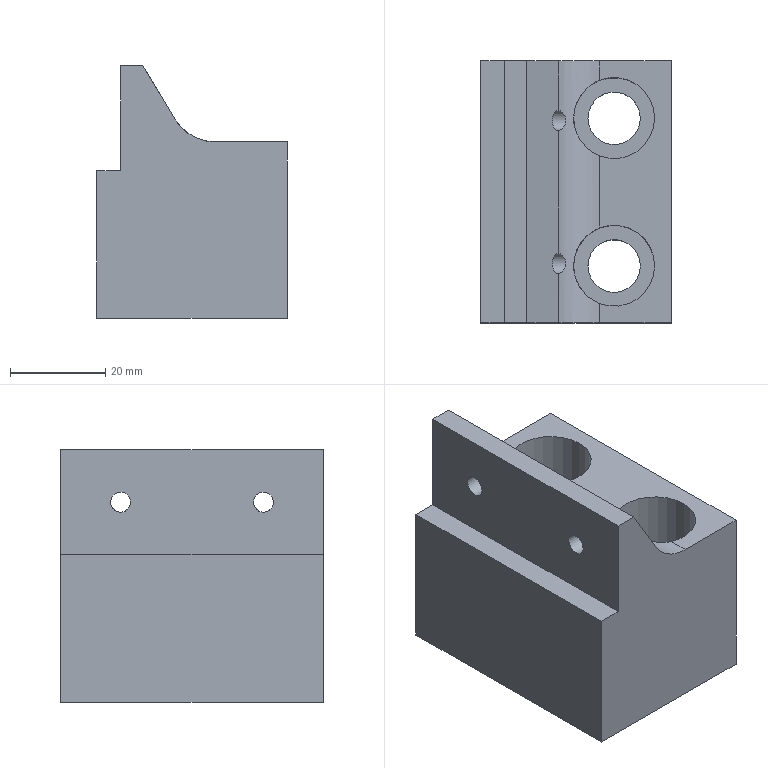Part | STEP file | 1 solid | 19 faces | box 40 x 55 x 53 mm | volume 73845 mm3 | plane 12 | cylinder 7 | commonest cylinder face diameters 4.2 x2 11 x2 17 x2 20 x1
STEP:
#1=CARTESIAN_POINT('',(132.93,-48.426,-20.));
#2=VERTEX_POINT('',#1);
#3=CARTESIAN_POINT('',(132.93,-32.574,-20.));
#4=VERTEX_POINT('',#3);
#5=CARTESIAN_POINT('',(136.,-40.5,-20.));
#6=DIRECTION('',(0.,0.,1.));
#7=DIRECTION('',(-1.,0.,0.));
#8=AXIS2_PLACEMENT_3D('',#5,#6,#7);
#9=CIRCLE('',#8,8.5);
#10=EDGE_CURVE('',#2,#4,#9,.T.);
#11=ORIENTED_EDGE('',*,*,#10,.F.);
#12=CARTESIAN_POINT('',(132.93,-63.574,-20.));
#13=VERTEX_POINT('',#12);
#14=CARTESIAN_POINT('',(132.93,-56.,-20.));
#15=DIRECTION('',(0.,-1.,0.));
#16=VECTOR('',#15,1.);
#17=LINE('',#14,#16);
#18=EDGE_CURVE('',#2,#13,#17,.T.);
#19=ORIENTED_EDGE('',*,*,#18,.T.);
#20=CARTESIAN_POINT('',(132.93,-79.426,-20.));
#21=VERTEX_POINT('',#20);
#22=CARTESIAN_POINT('',(136.,-71.5,-20.));
#23=DIRECTION('',(0.,0.,-1.));
#24=DIRECTION('',(-1.,0.,0.));
#25=AXIS2_PLACEMENT_3D('',#22,#23,#24);
#26=CIRCLE('',#25,8.5);
#27=EDGE_CURVE('',#13,#21,#26,.T.);
#28=ORIENTED_EDGE('',*,*,#27,.T.);
#29=CARTESIAN_POINT('',(132.93,-83.5,-20.));
#30=VERTEX_POINT('',#29);
#31=CARTESIAN_POINT('',(132.93,-56.,-20.));
#32=DIRECTION('',(0.,-1.,0.));
#33=VECTOR('',#32,1.);
#34=LINE('',#31,#33);
#35=EDGE_CURVE('',#21,#30,#34,.T.);
#36=ORIENTED_EDGE('',*,*,#35,.T.);
#37=CARTESIAN_POINT('',(148.,-83.5,-20.));
#38=VERTEX_POINT('',#37);
#39=CARTESIAN_POINT('',(106.5,-83.5,-20.));
#40=DIRECTION('',(-1.,0.,0.));
#41=VECTOR('',#40,1.);
#42=LINE('',#39,#41);
#43=EDGE_CURVE('',#38,#30,#42,.T.);
#44=ORIENTED_EDGE('',*,*,#43,.F.);
#45=CARTESIAN_POINT('',(148.,-28.5,-20.));
#46=VERTEX_POINT('',#45);
#47=CARTESIAN_POINT('',(148.,-56.,-20.));
#48=DIRECTION('',(0.,-1.,0.));
#49=VECTOR('',#48,1.);
#50=LINE('',#47,#49);
#51=EDGE_CURVE('',#46,#38,#50,.T.);
#52=ORIENTED_EDGE('',*,*,#51,.F.);
#53=CARTESIAN_POINT('',(132.93,-28.5,-20.));
#54=VERTEX_POINT('',#53);
#55=CARTESIAN_POINT('',(106.5,-28.5,-20.));
#56=DIRECTION('',(1.,0.,0.));
#57=VECTOR('',#56,1.);
#58=LINE('',#55,#57);
#59=EDGE_CURVE('',#54,#46,#58,.T.);
#60=ORIENTED_EDGE('',*,*,#59,.F.);
#61=CARTESIAN_POINT('',(132.93,-56.,-20.));
#62=DIRECTION('',(0.,-1.,0.));
#63=VECTOR('',#62,1.);
#64=LINE('',#61,#63);
#65=EDGE_CURVE('',#54,#4,#64,.T.);
#66=ORIENTED_EDGE('',*,*,#65,.T.);
#67=EDGE_LOOP('',(#11,#19,#28,#36,#44,#52,#60,#66));
#68=FACE_OUTER_BOUND('',#67,.T.);
#69=CARTESIAN_POINT('',(106.5,-56.,-20.));
#70=DIRECTION('',(0.,0.,-1.));
#71=DIRECTION('',(-1.,0.,0.));
#72=AXIS2_PLACEMENT_3D('',#69,#70,#71);
#73=PLANE('',#72);
#74=ADVANCED_FACE('',(#68),#73,.F.);
#75=ORIENTED_EDGE('',*,*,#51,.T.);
#76=CARTESIAN_POINT('',(148.,-83.5,-57.));
#77=VERTEX_POINT('',#76);
#78=CARTESIAN_POINT('',(148.,-83.5,-22.));
#79=DIRECTION('',(0.,0.,1.));
#80=VECTOR('',#79,1.);
#81=LINE('',#78,#80);
#82=EDGE_CURVE('',#77,#38,#81,.T.);
#83=ORIENTED_EDGE('',*,*,#82,.F.);
#84=CARTESIAN_POINT('',(148.,-28.5,-57.));
#85=VERTEX_POINT('',#84);
#86=CARTESIAN_POINT('',(148.,-55.25,-57.));
#87=DIRECTION('',(0.,1.,0.));
#88=VECTOR('',#87,1.);
#89=LINE('',#86,#88);
#90=EDGE_CURVE('',#77,#85,#89,.T.);
#91=ORIENTED_EDGE('',*,*,#90,.T.);
#92=CARTESIAN_POINT('',(148.,-28.5,-22.));
#93=DIRECTION('',(0.,0.,-1.));
#94=VECTOR('',#93,1.);
#95=LINE('',#92,#94);
#96=EDGE_CURVE('',#46,#85,#95,.T.);
#97=ORIENTED_EDGE('',*,*,#96,.F.);
#98=EDGE_LOOP('',(#75,#83,#91,#97));
#99=FACE_OUTER_BOUND('',#98,.T.);
#100=CARTESIAN_POINT('',(148.,-55.25,-43.5));
#101=DIRECTION('',(1.,0.,0.));
#102=DIRECTION('',(0.,0.,-1.));
#103=AXIS2_PLACEMENT_3D('',#100,#101,#102);
#104=PLANE('',#103);
#105=ADVANCED_FACE('',(#99),#104,.T.);
#106=CARTESIAN_POINT('',(124.355,-68.905,-15.145));
#107=VERTEX_POINT('',#106);
#108=CARTESIAN_POINT('',(124.355,-73.095,-15.145));
#109=VERTEX_POINT('',#108);
#110=CARTESIAN_POINT('',(124.268,-71.,-15.));
#111=DIRECTION('',(0.8575,0.,0.5145));
#112=DIRECTION('',(0.5145,0.,-0.8575));
#113=AXIS2_PLACEMENT_3D('',#110,#111,#112);
#114=ELLIPSE('',#113,2.449,2.1);
#115=EDGE_CURVE('',#107,#109,#114,.T.);
#116=ORIENTED_EDGE('',*,*,#115,.F.);
#117=CARTESIAN_POINT('',(124.355,-43.095,-15.145));
#118=VERTEX_POINT('',#117);
#119=CARTESIAN_POINT('',(124.355,-56.,-15.145));
#120=DIRECTION('',(0.,1.,0.));
#121=VECTOR('',#120,1.);
#122=LINE('',#119,#121);
#123=EDGE_CURVE('',#107,#118,#122,.T.);
#124=ORIENTED_EDGE('',*,*,#123,.T.);
#125=CARTESIAN_POINT('',(124.355,-38.905,-15.145));
#126=VERTEX_POINT('',#125);
#127=CARTESIAN_POINT('',(124.268,-41.,-15.));
#128=DIRECTION('',(0.8575,0.,0.5145));
#129=DIRECTION('',(0.5145,0.,-0.8575));
#130=AXIS2_PLACEMENT_3D('',#127,#128,#129);
#131=ELLIPSE('',#130,2.449,2.1);
#132=EDGE_CURVE('',#126,#118,#131,.T.);
#133=ORIENTED_EDGE('',*,*,#132,.F.);
#134=CARTESIAN_POINT('',(124.355,-28.5,-15.145));
#135=VERTEX_POINT('',#134);
#136=CARTESIAN_POINT('',(124.355,-56.,-15.145));
#137=DIRECTION('',(0.,1.,0.));
#138=VECTOR('',#137,1.);
#139=LINE('',#136,#138);
#140=EDGE_CURVE('',#126,#135,#139,.T.);
#141=ORIENTED_EDGE('',*,*,#140,.T.);
#142=CARTESIAN_POINT('',(117.668,-28.5,-4.));
#143=VERTEX_POINT('',#142);
#144=CARTESIAN_POINT('',(120.403,-28.5,-8.558));
#145=DIRECTION('',(0.5145,0.,-0.8575));
#146=VECTOR('',#145,1.);
#147=LINE('',#144,#146);
#148=EDGE_CURVE('',#143,#135,#147,.T.);
#149=ORIENTED_EDGE('',*,*,#148,.F.);
#150=CARTESIAN_POINT('',(117.668,-83.5,-4.));
#151=VERTEX_POINT('',#150);
#152=CARTESIAN_POINT('',(117.668,-56.,-4.));
#153=DIRECTION('',(0.,1.,0.));
#154=VECTOR('',#153,1.);
#155=LINE('',#152,#154);
#156=EDGE_CURVE('',#151,#143,#155,.T.);
#157=ORIENTED_EDGE('',*,*,#156,.F.);
#158=CARTESIAN_POINT('',(124.355,-83.5,-15.145));
#159=VERTEX_POINT('',#158);
#160=CARTESIAN_POINT('',(120.403,-83.5,-8.558));
#161=DIRECTION('',(-0.5145,0.,0.8575));
#162=VECTOR('',#161,1.);
#163=LINE('',#160,#162);
#164=EDGE_CURVE('',#159,#151,#163,.T.);
#165=ORIENTED_EDGE('',*,*,#164,.F.);
#166=CARTESIAN_POINT('',(124.355,-56.,-15.145));
#167=DIRECTION('',(0.,1.,0.));
#168=VECTOR('',#167,1.);
#169=LINE('',#166,#168);
#170=EDGE_CURVE('',#159,#109,#169,.T.);
#171=ORIENTED_EDGE('',*,*,#170,.T.);
#172=EDGE_LOOP('',(#116,#124,#133,#141,#149,#157,#165,#171));
#173=FACE_OUTER_BOUND('',#172,.T.);
#174=CARTESIAN_POINT('',(118.285,-56.,-5.029));
#175=DIRECTION('',(0.8575,0.,0.5145));
#176=DIRECTION('',(0.,-1.,0.));
#177=AXIS2_PLACEMENT_3D('',#174,#175,#176);
#178=PLANE('',#177);
#179=ADVANCED_FACE('',(#173),#178,.T.);
#180=CARTESIAN_POINT('',(108.,-28.5,-57.));
#181=VERTEX_POINT('',#180);
#182=CARTESIAN_POINT('',(98.,-28.5,-57.));
#183=DIRECTION('',(1.,0.,0.));
#184=VECTOR('',#183,1.);
#185=LINE('',#182,#184);
#186=EDGE_CURVE('',#181,#85,#185,.T.);
#187=ORIENTED_EDGE('',*,*,#186,.F.);
#188=CARTESIAN_POINT('',(108.,-28.5,-26.));
#189=VERTEX_POINT('',#188);
#190=CARTESIAN_POINT('',(108.,-28.5,-22.));
#191=DIRECTION('',(0.,0.,-1.));
#192=VECTOR('',#191,1.);
#193=LINE('',#190,#192);
#194=EDGE_CURVE('',#189,#181,#193,.T.);
#195=ORIENTED_EDGE('',*,*,#194,.F.);
#196=CARTESIAN_POINT('',(113.,-28.5,-26.));
#197=VERTEX_POINT('',#196);
#198=CARTESIAN_POINT('',(98.,-28.5,-26.));
#199=DIRECTION('',(-1.,0.,0.));
#200=VECTOR('',#199,1.);
#201=LINE('',#198,#200);
#202=EDGE_CURVE('',#197,#189,#201,.T.);
#203=ORIENTED_EDGE('',*,*,#202,.F.);
#204=CARTESIAN_POINT('',(113.,-28.5,-4.));
#205=VERTEX_POINT('',#204);
#206=CARTESIAN_POINT('',(113.,-28.5,-29.));
#207=DIRECTION('',(0.,0.,1.));
#208=VECTOR('',#207,1.);
#209=LINE('',#206,#208);
#210=EDGE_CURVE('',#197,#205,#209,.T.);
#211=ORIENTED_EDGE('',*,*,#210,.T.);
#212=CARTESIAN_POINT('',(106.5,-28.5,-4.));
#213=DIRECTION('',(1.,0.,0.));
#214=VECTOR('',#213,1.);
#215=LINE('',#212,#214);
#216=EDGE_CURVE('',#205,#143,#215,.T.);
#217=ORIENTED_EDGE('',*,*,#216,.T.);
#218=ORIENTED_EDGE('',*,*,#148,.T.);
#219=CARTESIAN_POINT('',(132.93,-28.5,-10.));
#220=DIRECTION('',(0.,-1.,0.));
#221=DIRECTION('',(0.,0.,-1.));
#222=AXIS2_PLACEMENT_3D('',#219,#220,#221);
#223=CIRCLE('',#222,10.);
#224=EDGE_CURVE('',#135,#54,#223,.T.);
#225=ORIENTED_EDGE('',*,*,#224,.T.);
#226=ORIENTED_EDGE('',*,*,#59,.T.);
#227=ORIENTED_EDGE('',*,*,#96,.T.);
#228=EDGE_LOOP('',(#187,#195,#203,#211,#217,#218,#225,#226,#227));
#229=FACE_OUTER_BOUND('',#228,.T.);
#230=CARTESIAN_POINT('',(98.,-28.5,-22.));
#231=DIRECTION('',(0.,-1.,0.));
#232=DIRECTION('',(0.,0.,-1.));
#233=AXIS2_PLACEMENT_3D('',#230,#231,#232);
#234=PLANE('',#233);
#235=ADVANCED_FACE('',(#229),#234,.F.);
#236=CARTESIAN_POINT('',(130.5,-40.5,-57.));
#237=VERTEX_POINT('',#236);
#238=CARTESIAN_POINT('',(136.,-40.5,-57.));
#239=DIRECTION('',(0.,0.,-1.));
#240=DIRECTION('',(-1.,0.,0.));
#241=AXIS2_PLACEMENT_3D('',#238,#239,#240);
#242=CIRCLE('',#241,5.5);
#243=EDGE_CURVE('',#237,#237,#242,.T.);
#244=ORIENTED_EDGE('',*,*,#243,.F.);
#245=EDGE_LOOP('',(#244));
#246=FACE_BOUND('',#245,.T.);
#247=CARTESIAN_POINT('',(130.5,-71.5,-57.));
#248=VERTEX_POINT('',#247);
#249=CARTESIAN_POINT('',(136.,-71.5,-57.));
#250=DIRECTION('',(0.,0.,1.));
#251=DIRECTION('',(-1.,0.,0.));
#252=AXIS2_PLACEMENT_3D('',#249,#250,#251);
#253=CIRCLE('',#252,5.5);
#254=EDGE_CURVE('',#248,#248,#253,.T.);
#255=ORIENTED_EDGE('',*,*,#254,.T.);
#256=EDGE_LOOP('',(#255));
#257=FACE_BOUND('',#256,.T.);
#258=CARTESIAN_POINT('',(108.,-83.5,-57.));
#259=VERTEX_POINT('',#258);
#260=CARTESIAN_POINT('',(98.,-83.5,-57.));
#261=DIRECTION('',(1.,0.,0.));
#262=VECTOR('',#261,1.);
#263=LINE('',#260,#262);
#264=EDGE_CURVE('',#259,#77,#263,.T.);
#265=ORIENTED_EDGE('',*,*,#264,.F.);
#266=CARTESIAN_POINT('',(108.,-55.25,-57.));
#267=DIRECTION('',(0.,1.,0.));
#268=VECTOR('',#267,1.);
#269=LINE('',#266,#268);
#270=EDGE_CURVE('',#259,#181,#269,.T.);
#271=ORIENTED_EDGE('',*,*,#270,.T.);
#272=ORIENTED_EDGE('',*,*,#186,.T.);
#273=ORIENTED_EDGE('',*,*,#90,.F.);
#274=EDGE_LOOP('',(#265,#271,#272,#273));
#275=FACE_BOUND('',#274,.T.);
#276=CARTESIAN_POINT('',(98.,-55.25,-57.));
#277=DIRECTION('',(0.,0.,-1.));
#278=DIRECTION('',(0.,1.,0.));
#279=AXIS2_PLACEMENT_3D('',#276,#277,#278);
#280=PLANE('',#279);
#281=ADVANCED_FACE('',(#246,#257,#275),#280,.T.);
#282=CARTESIAN_POINT('',(108.,-83.5,-26.));
#283=VERTEX_POINT('',#282);
#284=CARTESIAN_POINT('',(108.,-83.5,-22.));
#285=DIRECTION('',(0.,0.,1.));
#286=VECTOR('',#285,1.);
#287=LINE('',#284,#286);
#288=EDGE_CURVE('',#259,#283,#287,.T.);
#289=ORIENTED_EDGE('',*,*,#288,.F.);
#290=ORIENTED_EDGE('',*,*,#264,.T.);
#291=ORIENTED_EDGE('',*,*,#82,.T.);
#292=ORIENTED_EDGE('',*,*,#43,.T.);
#293=CARTESIAN_POINT('',(132.93,-83.5,-10.));
#294=DIRECTION('',(0.,1.,0.));
#295=DIRECTION('',(0.,0.,1.));
#296=AXIS2_PLACEMENT_3D('',#293,#294,#295);
#297=CIRCLE('',#296,10.);
#298=EDGE_CURVE('',#30,#159,#297,.T.);
#299=ORIENTED_EDGE('',*,*,#298,.T.);
#300=ORIENTED_EDGE('',*,*,#164,.T.);
#301=CARTESIAN_POINT('',(113.,-83.5,-4.));
#302=VERTEX_POINT('',#301);
#303=CARTESIAN_POINT('',(106.5,-83.5,-4.));
#304=DIRECTION('',(-1.,0.,0.));
#305=VECTOR('',#304,1.);
#306=LINE('',#303,#305);
#307=EDGE_CURVE('',#151,#302,#306,.T.);
#308=ORIENTED_EDGE('',*,*,#307,.T.);
#309=CARTESIAN_POINT('',(113.,-83.5,-26.));
#310=VERTEX_POINT('',#309);
#311=CARTESIAN_POINT('',(113.,-83.5,-29.));
#312=DIRECTION('',(0.,0.,1.));
#313=VECTOR('',#312,1.);
#314=LINE('',#311,#313);
#315=EDGE_CURVE('',#310,#302,#314,.T.);
#316=ORIENTED_EDGE('',*,*,#315,.F.);
#317=CARTESIAN_POINT('',(98.,-83.5,-26.));
#318=DIRECTION('',(1.,0.,0.));
#319=VECTOR('',#318,1.);
#320=LINE('',#317,#319);
#321=EDGE_CURVE('',#283,#310,#320,.T.);
#322=ORIENTED_EDGE('',*,*,#321,.F.);
#323=EDGE_LOOP('',(#289,#290,#291,#292,#299,#300,#308,#316,#322));
#324=FACE_OUTER_BOUND('',#323,.T.);
#325=CARTESIAN_POINT('',(98.,-83.5,-22.));
#326=DIRECTION('',(0.,1.,0.));
#327=DIRECTION('',(0.,0.,1.));
#328=AXIS2_PLACEMENT_3D('',#325,#326,#327);
#329=PLANE('',#328);
#330=ADVANCED_FACE('',(#324),#329,.F.);
#331=ORIENTED_EDGE('',*,*,#307,.F.);
#332=ORIENTED_EDGE('',*,*,#156,.T.);
#333=ORIENTED_EDGE('',*,*,#216,.F.);
#334=CARTESIAN_POINT('',(113.,-56.,-4.));
#335=DIRECTION('',(0.,-1.,0.));
#336=VECTOR('',#335,1.);
#337=LINE('',#334,#336);
#338=EDGE_CURVE('',#205,#302,#337,.T.);
#339=ORIENTED_EDGE('',*,*,#338,.T.);
#340=EDGE_LOOP('',(#331,#332,#333,#339));
#341=FACE_OUTER_BOUND('',#340,.T.);
#342=CARTESIAN_POINT('',(106.5,-56.,-4.));
#343=DIRECTION('',(0.,0.,-1.));
#344=DIRECTION('',(-1.,0.,0.));
#345=AXIS2_PLACEMENT_3D('',#342,#343,#344);
#346=PLANE('',#345);
#347=ADVANCED_FACE('',(#341),#346,.F.);
#348=ORIENTED_EDGE('',*,*,#288,.T.);
#349=CARTESIAN_POINT('',(108.,-55.25,-26.));
#350=DIRECTION('',(0.,1.,0.));
#351=VECTOR('',#350,1.);
#352=LINE('',#349,#351);
#353=EDGE_CURVE('',#283,#189,#352,.T.);
#354=ORIENTED_EDGE('',*,*,#353,.T.);
#355=ORIENTED_EDGE('',*,*,#194,.T.);
#356=ORIENTED_EDGE('',*,*,#270,.F.);
#357=EDGE_LOOP('',(#348,#354,#355,#356));
#358=FACE_OUTER_BOUND('',#357,.T.);
#359=CARTESIAN_POINT('',(108.,-55.25,-43.5));
#360=DIRECTION('',(1.,0.,0.));
#361=DIRECTION('',(0.,0.,-1.));
#362=AXIS2_PLACEMENT_3D('',#359,#360,#361);
#363=PLANE('',#362);
#364=ADVANCED_FACE('',(#358),#363,.F.);
#365=ORIENTED_EDGE('',*,*,#321,.T.);
#366=CARTESIAN_POINT('',(113.,-86.,-26.));
#367=DIRECTION('',(0.,-1.,0.));
#368=VECTOR('',#367,1.);
#369=LINE('',#366,#368);
#370=EDGE_CURVE('',#197,#310,#369,.T.);
#371=ORIENTED_EDGE('',*,*,#370,.F.);
#372=ORIENTED_EDGE('',*,*,#202,.T.);
#373=ORIENTED_EDGE('',*,*,#353,.F.);
#374=EDGE_LOOP('',(#365,#371,#372,#373));
#375=FACE_OUTER_BOUND('',#374,.T.);
#376=CARTESIAN_POINT('',(103.2,-86.,-26.));
#377=DIRECTION('',(0.,0.,1.));
#378=DIRECTION('',(1.,0.,0.));
#379=AXIS2_PLACEMENT_3D('',#376,#377,#378);
#380=PLANE('',#379);
#381=ADVANCED_FACE('',(#375),#380,.T.);
#382=ORIENTED_EDGE('',*,*,#370,.T.);
#383=ORIENTED_EDGE('',*,*,#315,.T.);
#384=ORIENTED_EDGE('',*,*,#338,.F.);
#385=ORIENTED_EDGE('',*,*,#210,.F.);
#386=EDGE_LOOP('',(#382,#383,#384,#385));
#387=FACE_BOUND('',#386,.T.);
#388=CARTESIAN_POINT('',(113.,-41.,-17.1));
#389=VERTEX_POINT('',#388);
#390=CARTESIAN_POINT('',(113.,-41.,-15.));
#391=DIRECTION('',(1.,0.,0.));
#392=DIRECTION('',(0.,0.,-1.));
#393=AXIS2_PLACEMENT_3D('',#390,#391,#392);
#394=CIRCLE('',#393,2.1);
#395=EDGE_CURVE('',#389,#389,#394,.T.);
#396=ORIENTED_EDGE('',*,*,#395,.T.);
#397=EDGE_LOOP('',(#396));
#398=FACE_BOUND('',#397,.T.);
#399=CARTESIAN_POINT('',(113.,-71.,-17.1));
#400=VERTEX_POINT('',#399);
#401=CARTESIAN_POINT('',(113.,-71.,-15.));
#402=DIRECTION('',(1.,0.,0.));
#403=DIRECTION('',(0.,0.,-1.));
#404=AXIS2_PLACEMENT_3D('',#401,#402,#403);
#405=CIRCLE('',#404,2.1);
#406=EDGE_CURVE('',#400,#400,#405,.T.);
#407=ORIENTED_EDGE('',*,*,#406,.T.);
#408=EDGE_LOOP('',(#407));
#409=FACE_BOUND('',#408,.T.);
#410=CARTESIAN_POINT('',(113.,-56.,-29.));
#411=DIRECTION('',(1.,0.,0.));
#412=DIRECTION('',(0.,0.,-1.));
#413=AXIS2_PLACEMENT_3D('',#410,#411,#412);
#414=PLANE('',#413);
#415=ADVANCED_FACE('',(#387,#398,#409),#414,.F.);
#416=ORIENTED_EDGE('',*,*,#18,.F.);
#417=CARTESIAN_POINT('',(132.93,-48.426,-20.));
#418=CARTESIAN_POINT('',(131.302,-47.796,-20.));
#419=CARTESIAN_POINT('',(129.944,-46.699,-19.6));
#420=CARTESIAN_POINT('',(128.035,-43.914,-18.782));
#421=CARTESIAN_POINT('',(127.503,-42.233,-18.4));
#422=CARTESIAN_POINT('',(127.497,-38.799,-18.396));
#423=CARTESIAN_POINT('',(128.035,-37.09,-18.781));
#424=CARTESIAN_POINT('',(129.931,-34.317,-19.595));
#425=CARTESIAN_POINT('',(131.301,-33.205,-20.));
#426=CARTESIAN_POINT('',(132.93,-32.574,-20.));
#427=B_SPLINE_CURVE_WITH_KNOTS('',3,(#417,#418,#419,#420,#421,#422,#423,#424,#425,#426),.UNSPECIFIED.,.F.,.F.,(4,2,2,2,4),(0.,0.25,0.5,0.75,1.),.UNSPECIFIED.);
#428=EDGE_CURVE('',#2,#4,#427,.T.);
#429=ORIENTED_EDGE('',*,*,#428,.T.);
#430=ORIENTED_EDGE('',*,*,#65,.F.);
#431=ORIENTED_EDGE('',*,*,#224,.F.);
#432=ORIENTED_EDGE('',*,*,#140,.F.);
#433=CARTESIAN_POINT('',(124.355,-38.905,-15.145));
#434=CARTESIAN_POINT('',(124.538,-38.926,-15.45));
#435=CARTESIAN_POINT('',(124.738,-39.014,-15.745));
#436=CARTESIAN_POINT('',(124.934,-39.157,-16.006));
#437=CARTESIAN_POINT('',(125.115,-39.288,-16.247));
#438=CARTESIAN_POINT('',(125.298,-39.469,-16.466));
#439=CARTESIAN_POINT('',(125.456,-39.694,-16.645));
#440=CARTESIAN_POINT('',(125.566,-39.85,-16.769));
#441=CARTESIAN_POINT('',(125.667,-40.031,-16.876));
#442=CARTESIAN_POINT('',(125.743,-40.231,-16.954));
#443=CARTESIAN_POINT('',(125.804,-40.391,-17.017));
#444=CARTESIAN_POINT('',(125.85,-40.566,-17.063));
#445=CARTESIAN_POINT('',(125.872,-40.746,-17.085));
#446=CARTESIAN_POINT('',(125.894,-40.926,-17.107));
#447=CARTESIAN_POINT('',(125.892,-41.115,-17.105));
#448=CARTESIAN_POINT('',(125.867,-41.294,-17.079));
#449=CARTESIAN_POINT('',(125.843,-41.458,-17.056));
#450=CARTESIAN_POINT('',(125.801,-41.618,-17.013));
#451=CARTESIAN_POINT('',(125.745,-41.764,-16.956));
#452=CARTESIAN_POINT('',(125.667,-41.972,-16.875));
#453=CARTESIAN_POINT('',(125.561,-42.16,-16.763));
#454=CARTESIAN_POINT('',(125.446,-42.32,-16.633));
#455=CARTESIAN_POINT('',(125.295,-42.532,-16.462));
#456=CARTESIAN_POINT('',(125.122,-42.704,-16.255));
#457=CARTESIAN_POINT('',(124.951,-42.831,-16.029));
#458=CARTESIAN_POINT('',(124.777,-42.96,-15.799));
#459=CARTESIAN_POINT('',(124.6,-43.046,-15.542));
#460=CARTESIAN_POINT('',(124.435,-43.082,-15.276));
#461=CARTESIAN_POINT('',(124.408,-43.088,-15.233));
#462=CARTESIAN_POINT('',(124.381,-43.092,-15.189));
#463=CARTESIAN_POINT('',(124.355,-43.095,-15.145));
#464=B_SPLINE_CURVE_WITH_KNOTS('',3,(#433,#434,#435,#436,#437,#438,#439,#440,#441,#442,#443,#444,#445,#446,#447,#448,#449,#450,#451,#452,#453,#454,#455,#456,#457,#458,#459,#460,#461,#462,#463),.UNSPECIFIED.,.F.,.F.,(4,3,3,3,3,3,3,3,3,3,4),(0.,0.1517,0.2913,0.3875,0.4645,0.542,0.6124,0.7125,0.8446,0.9785,1.),.UNSPECIFIED.);
#465=EDGE_CURVE('',#126,#118,#464,.T.);
#466=ORIENTED_EDGE('',*,*,#465,.T.);
#467=ORIENTED_EDGE('',*,*,#123,.F.);
#468=CARTESIAN_POINT('',(124.355,-68.905,-15.145));
#469=CARTESIAN_POINT('',(124.538,-68.926,-15.45));
#470=CARTESIAN_POINT('',(124.738,-69.014,-15.745));
#471=CARTESIAN_POINT('',(124.934,-69.157,-16.006));
#472=CARTESIAN_POINT('',(125.115,-69.288,-16.247));
#473=CARTESIAN_POINT('',(125.298,-69.469,-16.466));
#474=CARTESIAN_POINT('',(125.456,-69.694,-16.645));
#475=CARTESIAN_POINT('',(125.566,-69.85,-16.769));
#476=CARTESIAN_POINT('',(125.667,-70.031,-16.876));
#477=CARTESIAN_POINT('',(125.743,-70.231,-16.954));
#478=CARTESIAN_POINT('',(125.804,-70.391,-17.017));
#479=CARTESIAN_POINT('',(125.85,-70.566,-17.063));
#480=CARTESIAN_POINT('',(125.872,-70.746,-17.085));
#481=CARTESIAN_POINT('',(125.894,-70.926,-17.107));
#482=CARTESIAN_POINT('',(125.892,-71.115,-17.105));
#483=CARTESIAN_POINT('',(125.867,-71.294,-17.079));
#484=CARTESIAN_POINT('',(125.843,-71.458,-17.056));
#485=CARTESIAN_POINT('',(125.801,-71.618,-17.013));
#486=CARTESIAN_POINT('',(125.745,-71.764,-16.956));
#487=CARTESIAN_POINT('',(125.667,-71.972,-16.875));
#488=CARTESIAN_POINT('',(125.561,-72.16,-16.763));
#489=CARTESIAN_POINT('',(125.446,-72.32,-16.633));
#490=CARTESIAN_POINT('',(125.295,-72.532,-16.462));
#491=CARTESIAN_POINT('',(125.122,-72.704,-16.255));
#492=CARTESIAN_POINT('',(124.951,-72.831,-16.029));
#493=CARTESIAN_POINT('',(124.777,-72.96,-15.799));
#494=CARTESIAN_POINT('',(124.6,-73.046,-15.542));
#495=CARTESIAN_POINT('',(124.435,-73.082,-15.276));
#496=CARTESIAN_POINT('',(124.408,-73.088,-15.233));
#497=CARTESIAN_POINT('',(124.381,-73.092,-15.189));
#498=CARTESIAN_POINT('',(124.355,-73.095,-15.145));
#499=B_SPLINE_CURVE_WITH_KNOTS('',3,(#468,#469,#470,#471,#472,#473,#474,#475,#476,#477,#478,#479,#480,#481,#482,#483,#484,#485,#486,#487,#488,#489,#490,#491,#492,#493,#494,#495,#496,#497,#498),.UNSPECIFIED.,.F.,.F.,(4,3,3,3,3,3,3,3,3,3,4),(0.,0.1517,0.2913,0.3875,0.4645,0.542,0.6124,0.7125,0.8446,0.9785,1.),.UNSPECIFIED.);
#500=EDGE_CURVE('',#107,#109,#499,.T.);
#501=ORIENTED_EDGE('',*,*,#500,.T.);
#502=ORIENTED_EDGE('',*,*,#170,.F.);
#503=ORIENTED_EDGE('',*,*,#298,.F.);
#504=ORIENTED_EDGE('',*,*,#35,.F.);
#505=CARTESIAN_POINT('',(132.93,-79.426,-20.));
#506=CARTESIAN_POINT('',(131.302,-78.796,-20.));
#507=CARTESIAN_POINT('',(129.944,-77.699,-19.6));
#508=CARTESIAN_POINT('',(128.035,-74.914,-18.782));
#509=CARTESIAN_POINT('',(127.503,-73.233,-18.4));
#510=CARTESIAN_POINT('',(127.497,-69.799,-18.396));
#511=CARTESIAN_POINT('',(128.035,-68.09,-18.781));
#512=CARTESIAN_POINT('',(129.931,-65.317,-19.595));
#513=CARTESIAN_POINT('',(131.301,-64.205,-20.));
#514=CARTESIAN_POINT('',(132.93,-63.574,-20.));
#515=B_SPLINE_CURVE_WITH_KNOTS('',3,(#505,#506,#507,#508,#509,#510,#511,#512,#513,#514),.UNSPECIFIED.,.F.,.F.,(4,2,2,2,4),(0.,0.25,0.5,0.75,1.),.UNSPECIFIED.);
#516=EDGE_CURVE('',#21,#13,#515,.T.);
#517=ORIENTED_EDGE('',*,*,#516,.T.);
#518=EDGE_LOOP('',(#416,#429,#430,#431,#432,#466,#467,#501,#502,#503,#504,#517));
#519=FACE_OUTER_BOUND('',#518,.T.);
#520=CARTESIAN_POINT('',(132.93,-56.,-10.));
#521=DIRECTION('',(0.,-1.,0.));
#522=DIRECTION('',(0.,0.,-1.));
#523=AXIS2_PLACEMENT_3D('',#520,#521,#522);
#524=CYLINDRICAL_SURFACE('',#523,10.);
#525=ADVANCED_FACE('',(#519),#524,.F.);
#526=ORIENTED_EDGE('',*,*,#132,.T.);
#527=ORIENTED_EDGE('',*,*,#465,.F.);
#528=EDGE_LOOP('',(#526,#527));
#529=FACE_BOUND('',#528,.T.);
#530=ORIENTED_EDGE('',*,*,#395,.F.);
#531=EDGE_LOOP('',(#530));
#532=FACE_BOUND('',#531,.T.);
#533=CARTESIAN_POINT('',(113.,-41.,-15.));
#534=DIRECTION('',(1.,0.,0.));
#535=DIRECTION('',(0.,0.,1.));
#536=AXIS2_PLACEMENT_3D('',#533,#534,#535);
#537=CYLINDRICAL_SURFACE('',#536,2.1);
#538=ADVANCED_FACE('',(#529,#532),#537,.F.);
#539=ORIENTED_EDGE('',*,*,#115,.T.);
#540=ORIENTED_EDGE('',*,*,#500,.F.);
#541=EDGE_LOOP('',(#539,#540));
#542=FACE_BOUND('',#541,.T.);
#543=ORIENTED_EDGE('',*,*,#406,.F.);
#544=EDGE_LOOP('',(#543));
#545=FACE_BOUND('',#544,.T.);
#546=CARTESIAN_POINT('',(113.,-71.,-15.));
#547=DIRECTION('',(1.,0.,0.));
#548=DIRECTION('',(0.,0.,1.));
#549=AXIS2_PLACEMENT_3D('',#546,#547,#548);
#550=CYLINDRICAL_SURFACE('',#549,2.1);
#551=ADVANCED_FACE('',(#542,#545),#550,.F.);
#552=CARTESIAN_POINT('',(141.5,-71.5,-47.));
#553=VERTEX_POINT('',#552);
#554=CARTESIAN_POINT('',(136.,-71.5,-47.));
#555=DIRECTION('',(0.,0.,-1.));
#556=DIRECTION('',(1.,0.,0.));
#557=AXIS2_PLACEMENT_3D('',#554,#555,#556);
#558=CIRCLE('',#557,5.5);
#559=EDGE_CURVE('',#553,#553,#558,.T.);
#560=ORIENTED_EDGE('',*,*,#559,.F.);
#561=EDGE_LOOP('',(#560));
#562=FACE_BOUND('',#561,.T.);
#563=ORIENTED_EDGE('',*,*,#254,.F.);
#564=EDGE_LOOP('',(#563));
#565=FACE_BOUND('',#564,.T.);
#566=CARTESIAN_POINT('',(136.,-71.5,-57.));
#567=DIRECTION('',(0.,0.,1.));
#568=DIRECTION('',(-1.,0.,0.));
#569=AXIS2_PLACEMENT_3D('',#566,#567,#568);
#570=CYLINDRICAL_SURFACE('',#569,5.5);
#571=ADVANCED_FACE('',(#562,#565),#570,.F.);
#572=ORIENTED_EDGE('',*,*,#559,.T.);
#573=EDGE_LOOP('',(#572));
#574=FACE_BOUND('',#573,.T.);
#575=CARTESIAN_POINT('',(127.5,-71.5,-47.));
#576=VERTEX_POINT('',#575);
#577=CARTESIAN_POINT('',(136.,-71.5,-47.));
#578=DIRECTION('',(0.,0.,-1.));
#579=DIRECTION('',(-1.,0.,0.));
#580=AXIS2_PLACEMENT_3D('',#577,#578,#579);
#581=CIRCLE('',#580,8.5);
#582=EDGE_CURVE('',#576,#576,#581,.T.);
#583=ORIENTED_EDGE('',*,*,#582,.F.);
#584=EDGE_LOOP('',(#583));
#585=FACE_BOUND('',#584,.T.);
#586=CARTESIAN_POINT('',(136.,-71.5,-47.));
#587=DIRECTION('',(0.,0.,-1.));
#588=DIRECTION('',(1.,0.,0.));
#589=AXIS2_PLACEMENT_3D('',#586,#587,#588);
#590=PLANE('',#589);
#591=ADVANCED_FACE('',(#574,#585),#590,.F.);
#592=ORIENTED_EDGE('',*,*,#27,.F.);
#593=ORIENTED_EDGE('',*,*,#516,.F.);
#594=EDGE_LOOP('',(#592,#593));
#595=FACE_BOUND('',#594,.T.);
#596=ORIENTED_EDGE('',*,*,#582,.T.);
#597=EDGE_LOOP('',(#596));
#598=FACE_BOUND('',#597,.T.);
#599=CARTESIAN_POINT('',(136.,-71.5,-47.));
#600=DIRECTION('',(0.,0.,1.));
#601=DIRECTION('',(-1.,0.,0.));
#602=AXIS2_PLACEMENT_3D('',#599,#600,#601);
#603=CYLINDRICAL_SURFACE('',#602,8.5);
#604=ADVANCED_FACE('',(#595,#598),#603,.F.);
#605=CARTESIAN_POINT('',(141.5,-40.5,-47.));
#606=VERTEX_POINT('',#605);
#607=CARTESIAN_POINT('',(136.,-40.5,-47.));
#608=DIRECTION('',(0.,0.,1.));
#609=DIRECTION('',(1.,0.,0.));
#610=AXIS2_PLACEMENT_3D('',#607,#608,#609);
#611=CIRCLE('',#610,5.5);
#612=EDGE_CURVE('',#606,#606,#611,.T.);
#613=ORIENTED_EDGE('',*,*,#612,.T.);
#614=EDGE_LOOP('',(#613));
#615=FACE_BOUND('',#614,.T.);
#616=ORIENTED_EDGE('',*,*,#243,.T.);
#617=EDGE_LOOP('',(#616));
#618=FACE_BOUND('',#617,.T.);
#619=CARTESIAN_POINT('',(136.,-40.5,-57.));
#620=DIRECTION('',(0.,0.,1.));
#621=DIRECTION('',(-1.,0.,0.));
#622=AXIS2_PLACEMENT_3D('',#619,#620,#621);
#623=CYLINDRICAL_SURFACE('',#622,5.5);
#624=ADVANCED_FACE('',(#615,#618),#623,.F.);
#625=ORIENTED_EDGE('',*,*,#612,.F.);
#626=EDGE_LOOP('',(#625));
#627=FACE_BOUND('',#626,.T.);
#628=CARTESIAN_POINT('',(127.5,-40.5,-47.));
#629=VERTEX_POINT('',#628);
#630=CARTESIAN_POINT('',(136.,-40.5,-47.));
#631=DIRECTION('',(0.,0.,1.));
#632=DIRECTION('',(-1.,0.,0.));
#633=AXIS2_PLACEMENT_3D('',#630,#631,#632);
#634=CIRCLE('',#633,8.5);
#635=EDGE_CURVE('',#629,#629,#634,.T.);
#636=ORIENTED_EDGE('',*,*,#635,.T.);
#637=EDGE_LOOP('',(#636));
#638=FACE_BOUND('',#637,.T.);
#639=CARTESIAN_POINT('',(136.,-40.5,-47.));
#640=DIRECTION('',(0.,0.,-1.));
#641=DIRECTION('',(1.,0.,0.));
#642=AXIS2_PLACEMENT_3D('',#639,#640,#641);
#643=PLANE('',#642);
#644=ADVANCED_FACE('',(#627,#638),#643,.F.);
#645=ORIENTED_EDGE('',*,*,#10,.T.);
#646=ORIENTED_EDGE('',*,*,#428,.F.);
#647=EDGE_LOOP('',(#645,#646));
#648=FACE_BOUND('',#647,.T.);
#649=ORIENTED_EDGE('',*,*,#635,.F.);
#650=EDGE_LOOP('',(#649));
#651=FACE_BOUND('',#650,.T.);
#652=CARTESIAN_POINT('',(136.,-40.5,-47.));
#653=DIRECTION('',(0.,0.,1.));
#654=DIRECTION('',(-1.,0.,0.));
#655=AXIS2_PLACEMENT_3D('',#652,#653,#654);
#656=CYLINDRICAL_SURFACE('',#655,8.5);
#657=ADVANCED_FACE('',(#648,#651),#656,.F.);
#658=CLOSED_SHELL('',(#74,#105,#179,#235,#281,#330,#347,#364,#381,#415,#525,#538,#551,#571,#591,#604,#624,#644,#657));
#659=MANIFOLD_SOLID_BREP('',#658);
#660=(LENGTH_UNIT()NAMED_UNIT(*)SI_UNIT(.MILLI.,.METRE.));
#661=UNCERTAINTY_MEASURE_WITH_UNIT(LENGTH_MEASURE(0.0508),#660,'','');
#662=(NAMED_UNIT(*)PLANE_ANGLE_UNIT()SI_UNIT($,.RADIAN.));
#663=PLANE_ANGLE_MEASURE_WITH_UNIT(PLANE_ANGLE_MEASURE(0.01745),#662);
#664=DIMENSIONAL_EXPONENTS(0.,0.,0.,0.,0.,0.,0.);
#665=(CONVERSION_BASED_UNIT('DEGREE',#663)NAMED_UNIT(#664)PLANE_ANGLE_UNIT());
#666=(NAMED_UNIT(*)SI_UNIT($,.STERADIAN.)SOLID_ANGLE_UNIT());
#667=(GEOMETRIC_REPRESENTATION_CONTEXT(3)GLOBAL_UNCERTAINTY_ASSIGNED_CONTEXT((#661))GLOBAL_UNIT_ASSIGNED_CONTEXT((#660,#665,#666))REPRESENTATION_CONTEXT('',''));
#668=ADVANCED_BREP_SHAPE_REPRESENTATION('',(#659),#667);